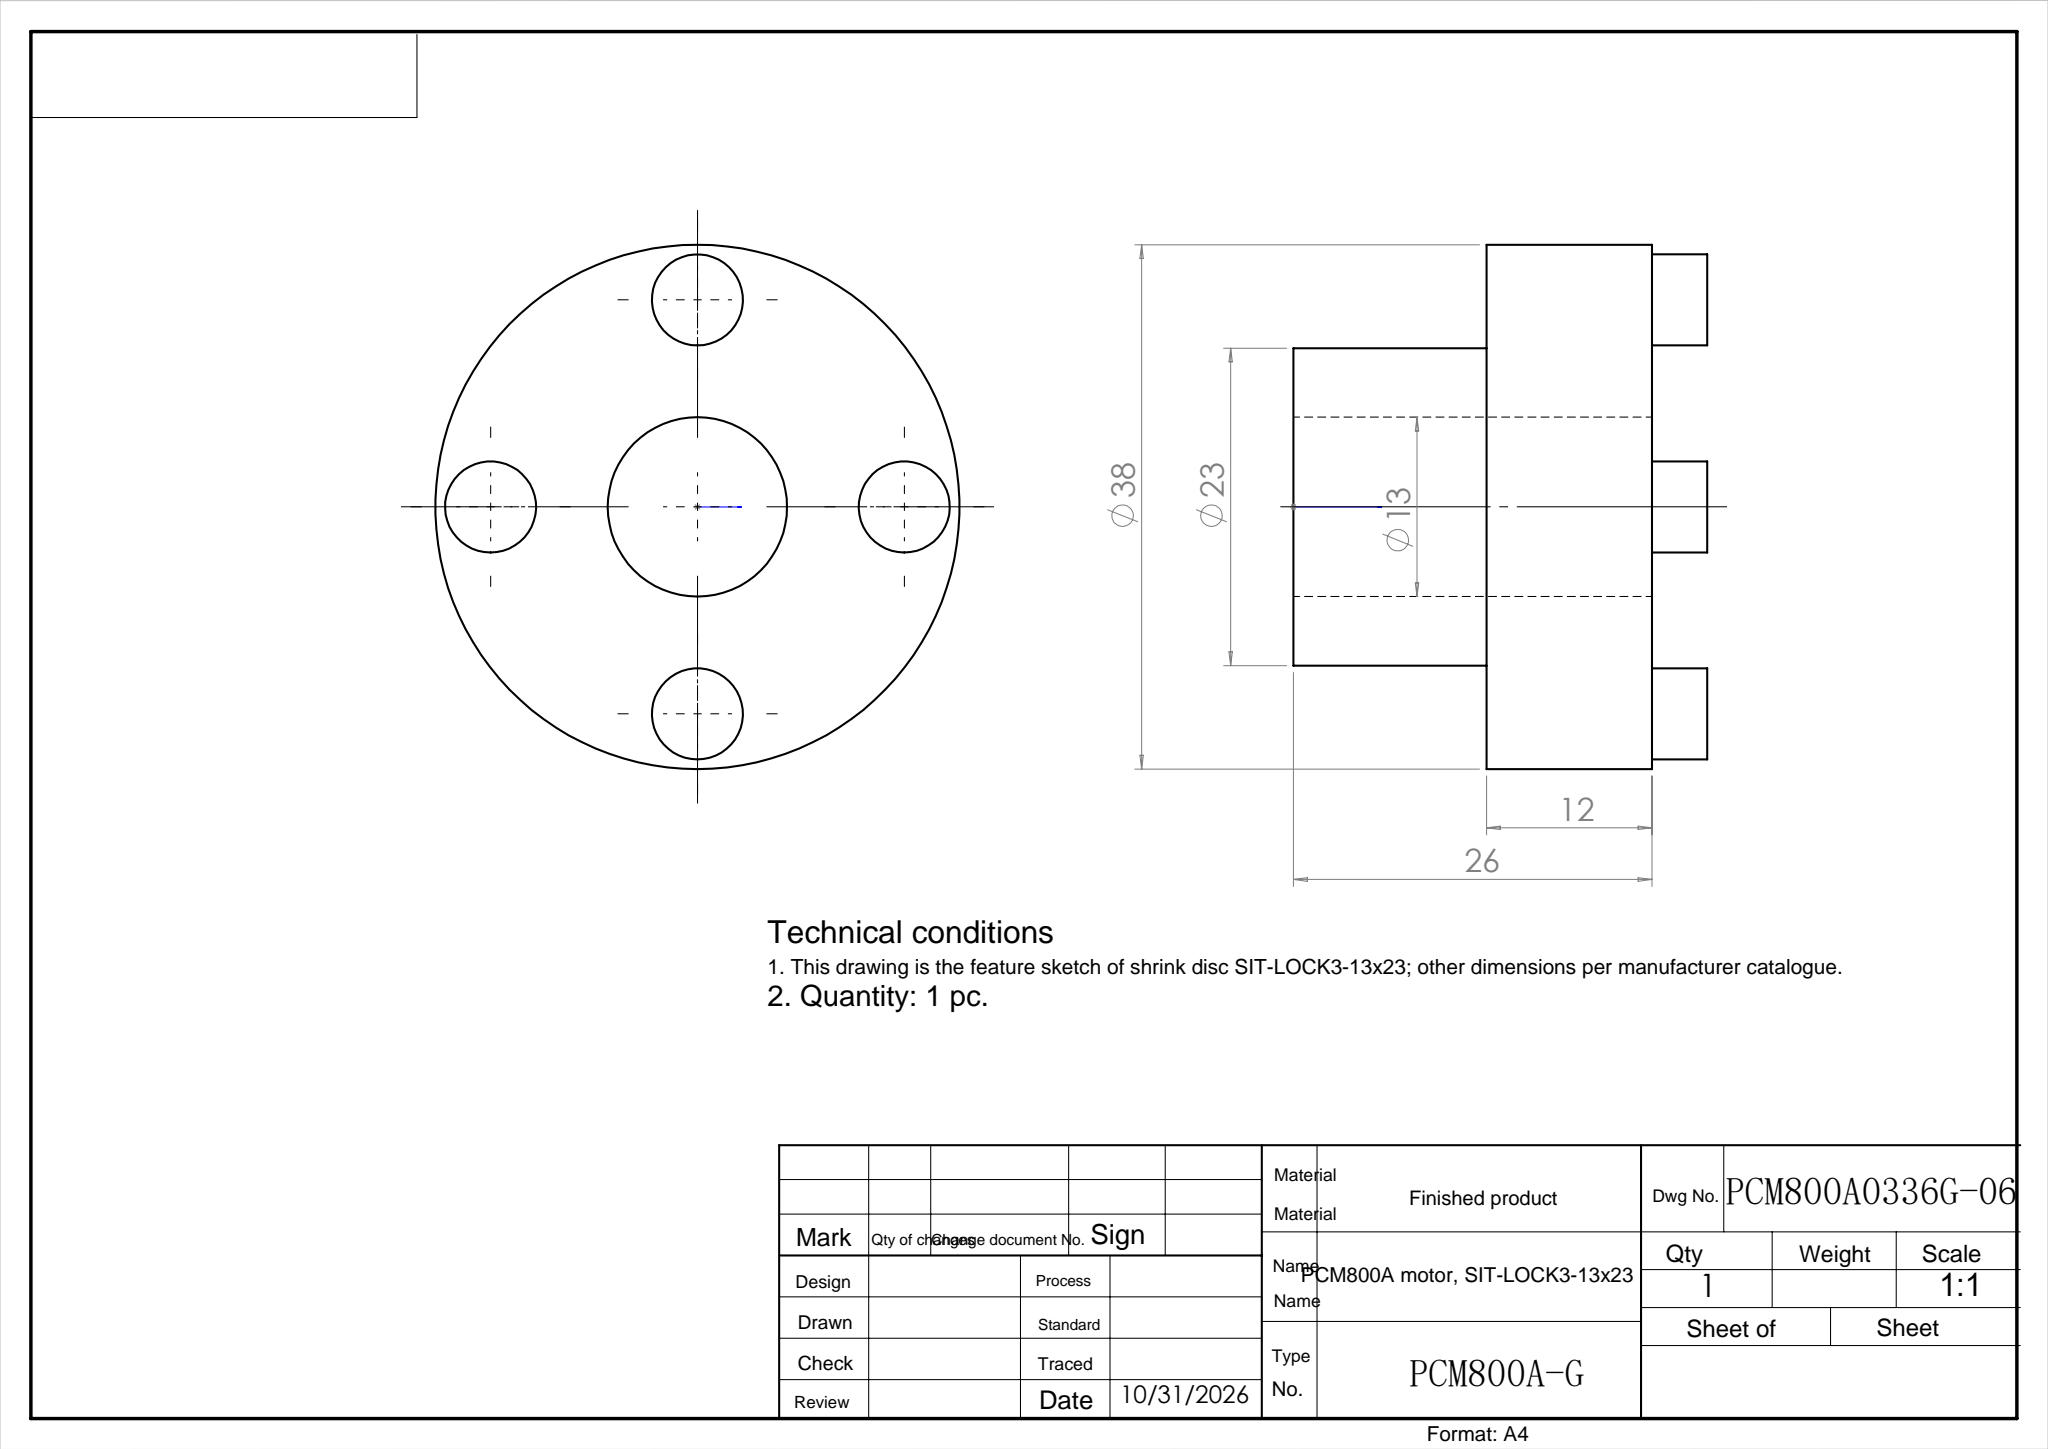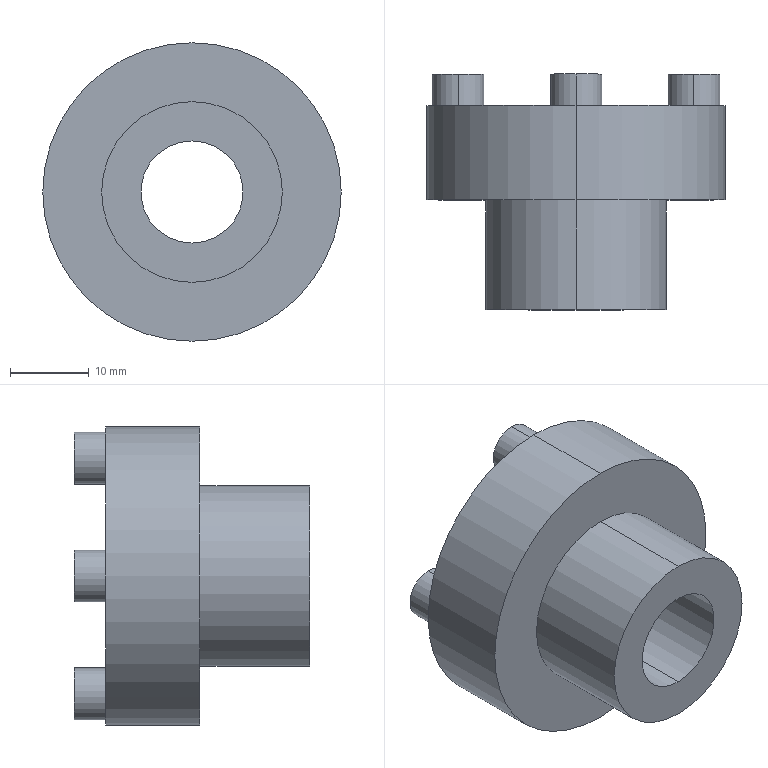Part | SolidWorks | features Boss 2, Extrusion 1 | 1 solid | 21 faces | box 38 x 30 x 38 mm | volume 16522 mm3 | cylinder 14 | plane 7 | commonest cylinder face diameters 6.6 x8 13 x2 23 x2 38 x2
STEP:
#1=CARTESIAN_POINT('',(-15.,30.,3.3));
#2=VERTEX_POINT('',#1);
#3=CARTESIAN_POINT('',(-15.,30.,-3.3));
#4=VERTEX_POINT('',#3);
#5=CARTESIAN_POINT('',(-15.,30.,0.));
#6=DIRECTION('',(0.,1.,0.));
#7=DIRECTION('',(0.,0.,1.));
#8=AXIS2_PLACEMENT_3D('',#5,#6,#7);
#9=CIRCLE('',#8,3.3);
#10=EDGE_CURVE('',#2,#4,#9,.T.);
#11=ORIENTED_EDGE('',*,*,#10,.F.);
#12=CARTESIAN_POINT('',(-15.,26.,3.3));
#13=VERTEX_POINT('',#12);
#14=CARTESIAN_POINT('',(-15.,30.,3.3));
#15=DIRECTION('',(0.,-1.,0.));
#16=VECTOR('',#15,1000.);
#17=LINE('',#14,#16);
#18=EDGE_CURVE('',#2,#13,#17,.T.);
#19=ORIENTED_EDGE('',*,*,#18,.T.);
#20=CARTESIAN_POINT('',(-15.,26.,-3.3));
#21=VERTEX_POINT('',#20);
#22=CARTESIAN_POINT('',(-15.,26.,0.));
#23=DIRECTION('',(0.,1.,0.));
#24=DIRECTION('',(0.,0.,1.));
#25=AXIS2_PLACEMENT_3D('',#22,#23,#24);
#26=CIRCLE('',#25,3.3);
#27=EDGE_CURVE('',#13,#21,#26,.T.);
#28=ORIENTED_EDGE('',*,*,#27,.T.);
#29=CARTESIAN_POINT('',(-15.,30.,-3.3));
#30=DIRECTION('',(0.,-1.,0.));
#31=VECTOR('',#30,1000.);
#32=LINE('',#29,#31);
#33=EDGE_CURVE('',#4,#21,#32,.T.);
#34=ORIENTED_EDGE('',*,*,#33,.F.);
#35=EDGE_LOOP('',(#11,#19,#28,#34));
#36=FACE_OUTER_BOUND('',#35,.T.);
#37=CARTESIAN_POINT('',(-15.,30.,0.));
#38=DIRECTION('',(0.,-1.,0.));
#39=DIRECTION('',(0.,0.,-1.));
#40=AXIS2_PLACEMENT_3D('',#37,#38,#39);
#41=CYLINDRICAL_SURFACE('',#40,3.3);
#42=ADVANCED_FACE('',(#36),#41,.T.);
#43=CARTESIAN_POINT('',(0.,30.,18.3));
#44=VERTEX_POINT('',#43);
#45=CARTESIAN_POINT('',(0.,30.,11.7));
#46=VERTEX_POINT('',#45);
#47=CARTESIAN_POINT('',(0.,30.,15.));
#48=DIRECTION('',(0.,1.,0.));
#49=DIRECTION('',(0.,0.,1.));
#50=AXIS2_PLACEMENT_3D('',#47,#48,#49);
#51=CIRCLE('',#50,3.3);
#52=EDGE_CURVE('',#44,#46,#51,.T.);
#53=ORIENTED_EDGE('',*,*,#52,.F.);
#54=CARTESIAN_POINT('',(0.,26.,18.3));
#55=VERTEX_POINT('',#54);
#56=CARTESIAN_POINT('',(0.,30.,18.3));
#57=DIRECTION('',(0.,-1.,0.));
#58=VECTOR('',#57,1000.);
#59=LINE('',#56,#58);
#60=EDGE_CURVE('',#44,#55,#59,.T.);
#61=ORIENTED_EDGE('',*,*,#60,.T.);
#62=CARTESIAN_POINT('',(0.,26.,11.7));
#63=VERTEX_POINT('',#62);
#64=CARTESIAN_POINT('',(0.,26.,15.));
#65=DIRECTION('',(0.,1.,0.));
#66=DIRECTION('',(0.,0.,1.));
#67=AXIS2_PLACEMENT_3D('',#64,#65,#66);
#68=CIRCLE('',#67,3.3);
#69=EDGE_CURVE('',#55,#63,#68,.T.);
#70=ORIENTED_EDGE('',*,*,#69,.T.);
#71=CARTESIAN_POINT('',(0.,30.,11.7));
#72=DIRECTION('',(0.,-1.,0.));
#73=VECTOR('',#72,1000.);
#74=LINE('',#71,#73);
#75=EDGE_CURVE('',#46,#63,#74,.T.);
#76=ORIENTED_EDGE('',*,*,#75,.F.);
#77=EDGE_LOOP('',(#53,#61,#70,#76));
#78=FACE_OUTER_BOUND('',#77,.T.);
#79=CARTESIAN_POINT('',(0.,30.,15.));
#80=DIRECTION('',(0.,-1.,0.));
#81=DIRECTION('',(0.,0.,-1.));
#82=AXIS2_PLACEMENT_3D('',#79,#80,#81);
#83=CYLINDRICAL_SURFACE('',#82,3.3);
#84=ADVANCED_FACE('',(#78),#83,.T.);
#85=CARTESIAN_POINT('',(0.,30.,-11.7));
#86=VERTEX_POINT('',#85);
#87=CARTESIAN_POINT('',(0.,30.,-18.3));
#88=VERTEX_POINT('',#87);
#89=CARTESIAN_POINT('',(0.,30.,-15.));
#90=DIRECTION('',(0.,1.,0.));
#91=DIRECTION('',(0.,0.,1.));
#92=AXIS2_PLACEMENT_3D('',#89,#90,#91);
#93=CIRCLE('',#92,3.3);
#94=EDGE_CURVE('',#86,#88,#93,.T.);
#95=ORIENTED_EDGE('',*,*,#94,.F.);
#96=CARTESIAN_POINT('',(0.,26.,-11.7));
#97=VERTEX_POINT('',#96);
#98=CARTESIAN_POINT('',(0.,30.,-11.7));
#99=DIRECTION('',(0.,-1.,0.));
#100=VECTOR('',#99,1000.);
#101=LINE('',#98,#100);
#102=EDGE_CURVE('',#86,#97,#101,.T.);
#103=ORIENTED_EDGE('',*,*,#102,.T.);
#104=CARTESIAN_POINT('',(0.,26.,-18.3));
#105=VERTEX_POINT('',#104);
#106=CARTESIAN_POINT('',(0.,26.,-15.));
#107=DIRECTION('',(0.,1.,0.));
#108=DIRECTION('',(0.,0.,1.));
#109=AXIS2_PLACEMENT_3D('',#106,#107,#108);
#110=CIRCLE('',#109,3.3);
#111=EDGE_CURVE('',#97,#105,#110,.T.);
#112=ORIENTED_EDGE('',*,*,#111,.T.);
#113=CARTESIAN_POINT('',(0.,30.,-18.3));
#114=DIRECTION('',(0.,-1.,0.));
#115=VECTOR('',#114,1000.);
#116=LINE('',#113,#115);
#117=EDGE_CURVE('',#88,#105,#116,.T.);
#118=ORIENTED_EDGE('',*,*,#117,.F.);
#119=EDGE_LOOP('',(#95,#103,#112,#118));
#120=FACE_OUTER_BOUND('',#119,.T.);
#121=CARTESIAN_POINT('',(0.,30.,-15.));
#122=DIRECTION('',(0.,-1.,0.));
#123=DIRECTION('',(0.,0.,-1.));
#124=AXIS2_PLACEMENT_3D('',#121,#122,#123);
#125=CYLINDRICAL_SURFACE('',#124,3.3);
#126=ADVANCED_FACE('',(#120),#125,.T.);
#127=CARTESIAN_POINT('',(15.,30.,3.3));
#128=VERTEX_POINT('',#127);
#129=CARTESIAN_POINT('',(15.,30.,-3.3));
#130=VERTEX_POINT('',#129);
#131=CARTESIAN_POINT('',(15.,30.,0.));
#132=DIRECTION('',(0.,1.,0.));
#133=DIRECTION('',(0.,0.,1.));
#134=AXIS2_PLACEMENT_3D('',#131,#132,#133);
#135=CIRCLE('',#134,3.3);
#136=EDGE_CURVE('',#128,#130,#135,.T.);
#137=ORIENTED_EDGE('',*,*,#136,.F.);
#138=CARTESIAN_POINT('',(15.,26.,3.3));
#139=VERTEX_POINT('',#138);
#140=CARTESIAN_POINT('',(15.,30.,3.3));
#141=DIRECTION('',(0.,-1.,0.));
#142=VECTOR('',#141,1000.);
#143=LINE('',#140,#142);
#144=EDGE_CURVE('',#128,#139,#143,.T.);
#145=ORIENTED_EDGE('',*,*,#144,.T.);
#146=CARTESIAN_POINT('',(15.,26.,-3.3));
#147=VERTEX_POINT('',#146);
#148=CARTESIAN_POINT('',(15.,26.,0.));
#149=DIRECTION('',(0.,1.,0.));
#150=DIRECTION('',(0.,0.,1.));
#151=AXIS2_PLACEMENT_3D('',#148,#149,#150);
#152=CIRCLE('',#151,3.3);
#153=EDGE_CURVE('',#139,#147,#152,.T.);
#154=ORIENTED_EDGE('',*,*,#153,.T.);
#155=CARTESIAN_POINT('',(15.,30.,-3.3));
#156=DIRECTION('',(0.,-1.,0.));
#157=VECTOR('',#156,1000.);
#158=LINE('',#155,#157);
#159=EDGE_CURVE('',#130,#147,#158,.T.);
#160=ORIENTED_EDGE('',*,*,#159,.F.);
#161=EDGE_LOOP('',(#137,#145,#154,#160));
#162=FACE_OUTER_BOUND('',#161,.T.);
#163=CARTESIAN_POINT('',(15.,30.,0.));
#164=DIRECTION('',(0.,-1.,0.));
#165=DIRECTION('',(0.,0.,-1.));
#166=AXIS2_PLACEMENT_3D('',#163,#164,#165);
#167=CYLINDRICAL_SURFACE('',#166,3.3);
#168=ADVANCED_FACE('',(#162),#167,.T.);
#169=CARTESIAN_POINT('',(0.,26.,19.));
#170=VERTEX_POINT('',#169);
#171=CARTESIAN_POINT('',(0.,26.,-19.));
#172=VERTEX_POINT('',#171);
#173=CARTESIAN_POINT('',(0.,26.,0.));
#174=DIRECTION('',(0.,1.,0.));
#175=DIRECTION('',(0.,0.,1.));
#176=AXIS2_PLACEMENT_3D('',#173,#174,#175);
#177=CIRCLE('',#176,19.);
#178=EDGE_CURVE('',#170,#172,#177,.T.);
#179=ORIENTED_EDGE('',*,*,#178,.F.);
#180=CARTESIAN_POINT('',(0.,14.,19.));
#181=VERTEX_POINT('',#180);
#182=CARTESIAN_POINT('',(0.,26.,19.));
#183=DIRECTION('',(0.,-1.,0.));
#184=VECTOR('',#183,1000.);
#185=LINE('',#182,#184);
#186=EDGE_CURVE('',#170,#181,#185,.T.);
#187=ORIENTED_EDGE('',*,*,#186,.T.);
#188=CARTESIAN_POINT('',(0.,14.,-19.));
#189=VERTEX_POINT('',#188);
#190=CARTESIAN_POINT('',(0.,14.,0.));
#191=DIRECTION('',(0.,1.,0.));
#192=DIRECTION('',(0.,0.,1.));
#193=AXIS2_PLACEMENT_3D('',#190,#191,#192);
#194=CIRCLE('',#193,19.);
#195=EDGE_CURVE('',#181,#189,#194,.T.);
#196=ORIENTED_EDGE('',*,*,#195,.T.);
#197=CARTESIAN_POINT('',(0.,26.,-19.));
#198=DIRECTION('',(0.,-1.,0.));
#199=VECTOR('',#198,1000.);
#200=LINE('',#197,#199);
#201=EDGE_CURVE('',#172,#189,#200,.T.);
#202=ORIENTED_EDGE('',*,*,#201,.F.);
#203=EDGE_LOOP('',(#179,#187,#196,#202));
#204=FACE_OUTER_BOUND('',#203,.T.);
#205=CARTESIAN_POINT('',(0.,26.,0.));
#206=DIRECTION('',(0.,-1.,0.));
#207=DIRECTION('',(0.,0.,-1.));
#208=AXIS2_PLACEMENT_3D('',#205,#206,#207);
#209=CYLINDRICAL_SURFACE('',#208,19.);
#210=ADVANCED_FACE('',(#204),#209,.T.);
#211=CARTESIAN_POINT('',(0.,26.,-6.5));
#212=VERTEX_POINT('',#211);
#213=CARTESIAN_POINT('',(0.,26.,6.5));
#214=VERTEX_POINT('',#213);
#215=CARTESIAN_POINT('',(0.,26.,0.));
#216=DIRECTION('',(0.,1.,0.));
#217=DIRECTION('',(0.,0.,1.));
#218=AXIS2_PLACEMENT_3D('',#215,#216,#217);
#219=CIRCLE('',#218,6.5);
#220=EDGE_CURVE('',#212,#214,#219,.T.);
#221=ORIENTED_EDGE('',*,*,#220,.T.);
#222=CARTESIAN_POINT('',(0.,0.,6.5));
#223=VERTEX_POINT('',#222);
#224=CARTESIAN_POINT('',(0.,14.,6.5));
#225=DIRECTION('',(0.,-1.,0.));
#226=VECTOR('',#225,1000.);
#227=LINE('',#224,#226);
#228=EDGE_CURVE('',#214,#223,#227,.T.);
#229=ORIENTED_EDGE('',*,*,#228,.T.);
#230=CARTESIAN_POINT('',(0.,0.,-6.5));
#231=VERTEX_POINT('',#230);
#232=CARTESIAN_POINT('',(0.,0.,0.));
#233=DIRECTION('',(0.,1.,0.));
#234=DIRECTION('',(0.,0.,1.));
#235=AXIS2_PLACEMENT_3D('',#232,#233,#234);
#236=CIRCLE('',#235,6.5);
#237=EDGE_CURVE('',#231,#223,#236,.T.);
#238=ORIENTED_EDGE('',*,*,#237,.F.);
#239=CARTESIAN_POINT('',(0.,14.,-6.5));
#240=DIRECTION('',(0.,-1.,0.));
#241=VECTOR('',#240,1000.);
#242=LINE('',#239,#241);
#243=EDGE_CURVE('',#212,#231,#242,.T.);
#244=ORIENTED_EDGE('',*,*,#243,.F.);
#245=EDGE_LOOP('',(#221,#229,#238,#244));
#246=FACE_OUTER_BOUND('',#245,.T.);
#247=CARTESIAN_POINT('',(0.,14.,0.));
#248=DIRECTION('',(0.,-1.,0.));
#249=DIRECTION('',(0.,0.,-1.));
#250=AXIS2_PLACEMENT_3D('',#247,#248,#249);
#251=CYLINDRICAL_SURFACE('',#250,6.5);
#252=ADVANCED_FACE('',(#246),#251,.F.);
#253=CARTESIAN_POINT('',(0.,14.,11.5));
#254=VERTEX_POINT('',#253);
#255=CARTESIAN_POINT('',(0.,14.,-11.5));
#256=VERTEX_POINT('',#255);
#257=CARTESIAN_POINT('',(0.,14.,0.));
#258=DIRECTION('',(0.,1.,0.));
#259=DIRECTION('',(0.,0.,1.));
#260=AXIS2_PLACEMENT_3D('',#257,#258,#259);
#261=CIRCLE('',#260,11.5);
#262=EDGE_CURVE('',#254,#256,#261,.T.);
#263=ORIENTED_EDGE('',*,*,#262,.F.);
#264=CARTESIAN_POINT('',(0.,0.,11.5));
#265=VERTEX_POINT('',#264);
#266=CARTESIAN_POINT('',(0.,14.,11.5));
#267=DIRECTION('',(0.,-1.,0.));
#268=VECTOR('',#267,1000.);
#269=LINE('',#266,#268);
#270=EDGE_CURVE('',#254,#265,#269,.T.);
#271=ORIENTED_EDGE('',*,*,#270,.T.);
#272=CARTESIAN_POINT('',(0.,0.,-11.5));
#273=VERTEX_POINT('',#272);
#274=CARTESIAN_POINT('',(0.,0.,0.));
#275=DIRECTION('',(0.,1.,0.));
#276=DIRECTION('',(0.,0.,1.));
#277=AXIS2_PLACEMENT_3D('',#274,#275,#276);
#278=CIRCLE('',#277,11.5);
#279=EDGE_CURVE('',#265,#273,#278,.T.);
#280=ORIENTED_EDGE('',*,*,#279,.T.);
#281=CARTESIAN_POINT('',(0.,14.,-11.5));
#282=DIRECTION('',(0.,-1.,0.));
#283=VECTOR('',#282,1000.);
#284=LINE('',#281,#283);
#285=EDGE_CURVE('',#256,#273,#284,.T.);
#286=ORIENTED_EDGE('',*,*,#285,.F.);
#287=EDGE_LOOP('',(#263,#271,#280,#286));
#288=FACE_OUTER_BOUND('',#287,.T.);
#289=CARTESIAN_POINT('',(0.,14.,0.));
#290=DIRECTION('',(0.,-1.,0.));
#291=DIRECTION('',(0.,0.,-1.));
#292=AXIS2_PLACEMENT_3D('',#289,#290,#291);
#293=CYLINDRICAL_SURFACE('',#292,11.5);
#294=ADVANCED_FACE('',(#288),#293,.T.);
#295=CARTESIAN_POINT('',(0.,26.,15.));
#296=DIRECTION('',(0.,1.,0.));
#297=DIRECTION('',(0.,0.,1.));
#298=AXIS2_PLACEMENT_3D('',#295,#296,#297);
#299=CIRCLE('',#298,3.3);
#300=EDGE_CURVE('',#63,#55,#299,.T.);
#301=ORIENTED_EDGE('',*,*,#300,.F.);
#302=ORIENTED_EDGE('',*,*,#69,.F.);
#303=EDGE_LOOP('',(#301,#302));
#304=FACE_BOUND('',#303,.T.);
#305=CARTESIAN_POINT('',(15.,26.,0.));
#306=DIRECTION('',(0.,1.,0.));
#307=DIRECTION('',(0.,0.,1.));
#308=AXIS2_PLACEMENT_3D('',#305,#306,#307);
#309=CIRCLE('',#308,3.3);
#310=EDGE_CURVE('',#147,#139,#309,.T.);
#311=ORIENTED_EDGE('',*,*,#310,.F.);
#312=ORIENTED_EDGE('',*,*,#153,.F.);
#313=EDGE_LOOP('',(#311,#312));
#314=FACE_BOUND('',#313,.T.);
#315=CARTESIAN_POINT('',(0.,26.,0.));
#316=DIRECTION('',(0.,1.,0.));
#317=DIRECTION('',(0.,0.,1.));
#318=AXIS2_PLACEMENT_3D('',#315,#316,#317);
#319=CIRCLE('',#318,19.);
#320=EDGE_CURVE('',#172,#170,#319,.T.);
#321=ORIENTED_EDGE('',*,*,#320,.T.);
#322=ORIENTED_EDGE('',*,*,#178,.T.);
#323=EDGE_LOOP('',(#321,#322));
#324=FACE_OUTER_BOUND('',#323,.T.);
#325=ORIENTED_EDGE('',*,*,#220,.F.);
#326=CARTESIAN_POINT('',(0.,26.,0.));
#327=DIRECTION('',(0.,1.,0.));
#328=DIRECTION('',(0.,0.,1.));
#329=AXIS2_PLACEMENT_3D('',#326,#327,#328);
#330=CIRCLE('',#329,6.5);
#331=EDGE_CURVE('',#214,#212,#330,.T.);
#332=ORIENTED_EDGE('',*,*,#331,.F.);
#333=EDGE_LOOP('',(#325,#332));
#334=FACE_BOUND('',#333,.T.);
#335=CARTESIAN_POINT('',(0.,26.,-15.));
#336=DIRECTION('',(0.,1.,0.));
#337=DIRECTION('',(0.,0.,1.));
#338=AXIS2_PLACEMENT_3D('',#335,#336,#337);
#339=CIRCLE('',#338,3.3);
#340=EDGE_CURVE('',#105,#97,#339,.T.);
#341=ORIENTED_EDGE('',*,*,#340,.F.);
#342=ORIENTED_EDGE('',*,*,#111,.F.);
#343=EDGE_LOOP('',(#341,#342));
#344=FACE_BOUND('',#343,.T.);
#345=CARTESIAN_POINT('',(-15.,26.,0.));
#346=DIRECTION('',(0.,1.,0.));
#347=DIRECTION('',(0.,0.,1.));
#348=AXIS2_PLACEMENT_3D('',#345,#346,#347);
#349=CIRCLE('',#348,3.3);
#350=EDGE_CURVE('',#21,#13,#349,.T.);
#351=ORIENTED_EDGE('',*,*,#350,.F.);
#352=ORIENTED_EDGE('',*,*,#27,.F.);
#353=EDGE_LOOP('',(#351,#352));
#354=FACE_BOUND('',#353,.T.);
#355=CARTESIAN_POINT('',(0.,26.,0.));
#356=DIRECTION('',(0.,1.,0.));
#357=DIRECTION('',(0.,0.,1.));
#358=AXIS2_PLACEMENT_3D('',#355,#356,#357);
#359=PLANE('',#358);
#360=ADVANCED_FACE('',(#304,#314,#324,#334,#344,#354),#359,.T.);
#361=CARTESIAN_POINT('',(0.,0.,0.));
#362=DIRECTION('',(0.,1.,0.));
#363=DIRECTION('',(0.,0.,1.));
#364=AXIS2_PLACEMENT_3D('',#361,#362,#363);
#365=CIRCLE('',#364,11.5);
#366=EDGE_CURVE('',#273,#265,#365,.T.);
#367=ORIENTED_EDGE('',*,*,#366,.F.);
#368=ORIENTED_EDGE('',*,*,#279,.F.);
#369=EDGE_LOOP('',(#367,#368));
#370=FACE_OUTER_BOUND('',#369,.T.);
#371=ORIENTED_EDGE('',*,*,#237,.T.);
#372=CARTESIAN_POINT('',(0.,0.,0.));
#373=DIRECTION('',(0.,1.,0.));
#374=DIRECTION('',(0.,0.,1.));
#375=AXIS2_PLACEMENT_3D('',#372,#373,#374);
#376=CIRCLE('',#375,6.5);
#377=EDGE_CURVE('',#223,#231,#376,.T.);
#378=ORIENTED_EDGE('',*,*,#377,.T.);
#379=EDGE_LOOP('',(#371,#378));
#380=FACE_BOUND('',#379,.T.);
#381=CARTESIAN_POINT('',(0.,0.,0.));
#382=DIRECTION('',(0.,1.,0.));
#383=DIRECTION('',(0.,0.,1.));
#384=AXIS2_PLACEMENT_3D('',#381,#382,#383);
#385=PLANE('',#384);
#386=ADVANCED_FACE('',(#370,#380),#385,.F.);
#387=ORIENTED_EDGE('',*,*,#270,.F.);
#388=CARTESIAN_POINT('',(0.,14.,0.));
#389=DIRECTION('',(0.,1.,0.));
#390=DIRECTION('',(0.,0.,1.));
#391=AXIS2_PLACEMENT_3D('',#388,#389,#390);
#392=CIRCLE('',#391,11.5);
#393=EDGE_CURVE('',#256,#254,#392,.T.);
#394=ORIENTED_EDGE('',*,*,#393,.F.);
#395=ORIENTED_EDGE('',*,*,#285,.T.);
#396=ORIENTED_EDGE('',*,*,#366,.T.);
#397=EDGE_LOOP('',(#387,#394,#395,#396));
#398=FACE_OUTER_BOUND('',#397,.T.);
#399=CARTESIAN_POINT('',(0.,14.,0.));
#400=DIRECTION('',(0.,-1.,0.));
#401=DIRECTION('',(0.,0.,-1.));
#402=AXIS2_PLACEMENT_3D('',#399,#400,#401);
#403=CYLINDRICAL_SURFACE('',#402,11.5);
#404=ADVANCED_FACE('',(#398),#403,.T.);
#405=ORIENTED_EDGE('',*,*,#228,.F.);
#406=ORIENTED_EDGE('',*,*,#331,.T.);
#407=ORIENTED_EDGE('',*,*,#243,.T.);
#408=ORIENTED_EDGE('',*,*,#377,.F.);
#409=EDGE_LOOP('',(#405,#406,#407,#408));
#410=FACE_OUTER_BOUND('',#409,.T.);
#411=CARTESIAN_POINT('',(0.,14.,0.));
#412=DIRECTION('',(0.,-1.,0.));
#413=DIRECTION('',(0.,0.,-1.));
#414=AXIS2_PLACEMENT_3D('',#411,#412,#413);
#415=CYLINDRICAL_SURFACE('',#414,6.5);
#416=ADVANCED_FACE('',(#410),#415,.F.);
#417=CARTESIAN_POINT('',(0.,14.,0.));
#418=DIRECTION('',(0.,1.,0.));
#419=DIRECTION('',(0.,0.,1.));
#420=AXIS2_PLACEMENT_3D('',#417,#418,#419);
#421=CIRCLE('',#420,19.);
#422=EDGE_CURVE('',#189,#181,#421,.T.);
#423=ORIENTED_EDGE('',*,*,#422,.F.);
#424=ORIENTED_EDGE('',*,*,#195,.F.);
#425=EDGE_LOOP('',(#423,#424));
#426=FACE_OUTER_BOUND('',#425,.T.);
#427=ORIENTED_EDGE('',*,*,#393,.T.);
#428=ORIENTED_EDGE('',*,*,#262,.T.);
#429=EDGE_LOOP('',(#427,#428));
#430=FACE_BOUND('',#429,.T.);
#431=CARTESIAN_POINT('',(0.,14.,0.));
#432=DIRECTION('',(0.,1.,0.));
#433=DIRECTION('',(0.,0.,1.));
#434=AXIS2_PLACEMENT_3D('',#431,#432,#433);
#435=PLANE('',#434);
#436=ADVANCED_FACE('',(#426,#430),#435,.F.);
#437=ORIENTED_EDGE('',*,*,#186,.F.);
#438=ORIENTED_EDGE('',*,*,#320,.F.);
#439=ORIENTED_EDGE('',*,*,#201,.T.);
#440=ORIENTED_EDGE('',*,*,#422,.T.);
#441=EDGE_LOOP('',(#437,#438,#439,#440));
#442=FACE_OUTER_BOUND('',#441,.T.);
#443=CARTESIAN_POINT('',(0.,26.,0.));
#444=DIRECTION('',(0.,-1.,0.));
#445=DIRECTION('',(0.,0.,-1.));
#446=AXIS2_PLACEMENT_3D('',#443,#444,#445);
#447=CYLINDRICAL_SURFACE('',#446,19.);
#448=ADVANCED_FACE('',(#442),#447,.T.);
#449=ORIENTED_EDGE('',*,*,#144,.F.);
#450=CARTESIAN_POINT('',(15.,30.,0.));
#451=DIRECTION('',(0.,1.,0.));
#452=DIRECTION('',(0.,0.,1.));
#453=AXIS2_PLACEMENT_3D('',#450,#451,#452);
#454=CIRCLE('',#453,3.3);
#455=EDGE_CURVE('',#130,#128,#454,.T.);
#456=ORIENTED_EDGE('',*,*,#455,.F.);
#457=ORIENTED_EDGE('',*,*,#159,.T.);
#458=ORIENTED_EDGE('',*,*,#310,.T.);
#459=EDGE_LOOP('',(#449,#456,#457,#458));
#460=FACE_OUTER_BOUND('',#459,.T.);
#461=CARTESIAN_POINT('',(15.,30.,0.));
#462=DIRECTION('',(0.,-1.,0.));
#463=DIRECTION('',(0.,0.,-1.));
#464=AXIS2_PLACEMENT_3D('',#461,#462,#463);
#465=CYLINDRICAL_SURFACE('',#464,3.3);
#466=ADVANCED_FACE('',(#460),#465,.T.);
#467=ORIENTED_EDGE('',*,*,#455,.T.);
#468=ORIENTED_EDGE('',*,*,#136,.T.);
#469=EDGE_LOOP('',(#467,#468));
#470=FACE_OUTER_BOUND('',#469,.T.);
#471=CARTESIAN_POINT('',(15.,30.,0.));
#472=DIRECTION('',(0.,1.,0.));
#473=DIRECTION('',(0.,0.,1.));
#474=AXIS2_PLACEMENT_3D('',#471,#472,#473);
#475=PLANE('',#474);
#476=ADVANCED_FACE('',(#470),#475,.T.);
#477=ORIENTED_EDGE('',*,*,#102,.F.);
#478=CARTESIAN_POINT('',(0.,30.,-15.));
#479=DIRECTION('',(0.,1.,0.));
#480=DIRECTION('',(0.,0.,1.));
#481=AXIS2_PLACEMENT_3D('',#478,#479,#480);
#482=CIRCLE('',#481,3.3);
#483=EDGE_CURVE('',#88,#86,#482,.T.);
#484=ORIENTED_EDGE('',*,*,#483,.F.);
#485=ORIENTED_EDGE('',*,*,#117,.T.);
#486=ORIENTED_EDGE('',*,*,#340,.T.);
#487=EDGE_LOOP('',(#477,#484,#485,#486));
#488=FACE_OUTER_BOUND('',#487,.T.);
#489=CARTESIAN_POINT('',(0.,30.,-15.));
#490=DIRECTION('',(0.,-1.,0.));
#491=DIRECTION('',(0.,0.,-1.));
#492=AXIS2_PLACEMENT_3D('',#489,#490,#491);
#493=CYLINDRICAL_SURFACE('',#492,3.3);
#494=ADVANCED_FACE('',(#488),#493,.T.);
#495=ORIENTED_EDGE('',*,*,#483,.T.);
#496=ORIENTED_EDGE('',*,*,#94,.T.);
#497=EDGE_LOOP('',(#495,#496));
#498=FACE_OUTER_BOUND('',#497,.T.);
#499=CARTESIAN_POINT('',(0.,30.,-15.));
#500=DIRECTION('',(0.,1.,0.));
#501=DIRECTION('',(0.,0.,1.));
#502=AXIS2_PLACEMENT_3D('',#499,#500,#501);
#503=PLANE('',#502);
#504=ADVANCED_FACE('',(#498),#503,.T.);
#505=ORIENTED_EDGE('',*,*,#60,.F.);
#506=CARTESIAN_POINT('',(0.,30.,15.));
#507=DIRECTION('',(0.,1.,0.));
#508=DIRECTION('',(0.,0.,1.));
#509=AXIS2_PLACEMENT_3D('',#506,#507,#508);
#510=CIRCLE('',#509,3.3);
#511=EDGE_CURVE('',#46,#44,#510,.T.);
#512=ORIENTED_EDGE('',*,*,#511,.F.);
#513=ORIENTED_EDGE('',*,*,#75,.T.);
#514=ORIENTED_EDGE('',*,*,#300,.T.);
#515=EDGE_LOOP('',(#505,#512,#513,#514));
#516=FACE_OUTER_BOUND('',#515,.T.);
#517=CARTESIAN_POINT('',(0.,30.,15.));
#518=DIRECTION('',(0.,-1.,0.));
#519=DIRECTION('',(0.,0.,-1.));
#520=AXIS2_PLACEMENT_3D('',#517,#518,#519);
#521=CYLINDRICAL_SURFACE('',#520,3.3);
#522=ADVANCED_FACE('',(#516),#521,.T.);
#523=ORIENTED_EDGE('',*,*,#511,.T.);
#524=ORIENTED_EDGE('',*,*,#52,.T.);
#525=EDGE_LOOP('',(#523,#524));
#526=FACE_OUTER_BOUND('',#525,.T.);
#527=CARTESIAN_POINT('',(0.,30.,15.));
#528=DIRECTION('',(0.,1.,0.));
#529=DIRECTION('',(0.,0.,1.));
#530=AXIS2_PLACEMENT_3D('',#527,#528,#529);
#531=PLANE('',#530);
#532=ADVANCED_FACE('',(#526),#531,.T.);
#533=ORIENTED_EDGE('',*,*,#18,.F.);
#534=CARTESIAN_POINT('',(-15.,30.,0.));
#535=DIRECTION('',(0.,1.,0.));
#536=DIRECTION('',(0.,0.,1.));
#537=AXIS2_PLACEMENT_3D('',#534,#535,#536);
#538=CIRCLE('',#537,3.3);
#539=EDGE_CURVE('',#4,#2,#538,.T.);
#540=ORIENTED_EDGE('',*,*,#539,.F.);
#541=ORIENTED_EDGE('',*,*,#33,.T.);
#542=ORIENTED_EDGE('',*,*,#350,.T.);
#543=EDGE_LOOP('',(#533,#540,#541,#542));
#544=FACE_OUTER_BOUND('',#543,.T.);
#545=CARTESIAN_POINT('',(-15.,30.,0.));
#546=DIRECTION('',(0.,-1.,0.));
#547=DIRECTION('',(0.,0.,-1.));
#548=AXIS2_PLACEMENT_3D('',#545,#546,#547);
#549=CYLINDRICAL_SURFACE('',#548,3.3);
#550=ADVANCED_FACE('',(#544),#549,.T.);
#551=ORIENTED_EDGE('',*,*,#539,.T.);
#552=ORIENTED_EDGE('',*,*,#10,.T.);
#553=EDGE_LOOP('',(#551,#552));
#554=FACE_OUTER_BOUND('',#553,.T.);
#555=CARTESIAN_POINT('',(-15.,30.,0.));
#556=DIRECTION('',(0.,1.,0.));
#557=DIRECTION('',(0.,0.,1.));
#558=AXIS2_PLACEMENT_3D('',#555,#556,#557);
#559=PLANE('',#558);
#560=ADVANCED_FACE('',(#554),#559,.T.);
#561=CLOSED_SHELL('',(#42,#84,#126,#168,#210,#252,#294,#360,#386,#404,#416,#436,#448,#466,#476,#494,#504,#522,#532,#550,#560));
#562=MANIFOLD_SOLID_BREP('',#561);
#563=CARTESIAN_POINT('',(0.,0.,0.));
#564=DIRECTION('',(0.,0.,1.));
#565=DIRECTION('',(1.,0.,0.));
#566=AXIS2_PLACEMENT_3D('',#563,#564,#565);
#567=(LENGTH_UNIT()NAMED_UNIT(*)SI_UNIT(.MILLI.,.METRE.));
#568=UNCERTAINTY_MEASURE_WITH_UNIT(LENGTH_MEASURE(0.00001),#567,'','');
#569=(NAMED_UNIT(*)PLANE_ANGLE_UNIT()SI_UNIT($,.RADIAN.));
#570=(NAMED_UNIT(*)SI_UNIT($,.STERADIAN.)SOLID_ANGLE_UNIT());
#571=(GEOMETRIC_REPRESENTATION_CONTEXT(3)GLOBAL_UNCERTAINTY_ASSIGNED_CONTEXT((#568))GLOBAL_UNIT_ASSIGNED_CONTEXT((#567,#569,#570))REPRESENTATION_CONTEXT('',''));
#572=ADVANCED_BREP_SHAPE_REPRESENTATION('',(#562,#566),#571);